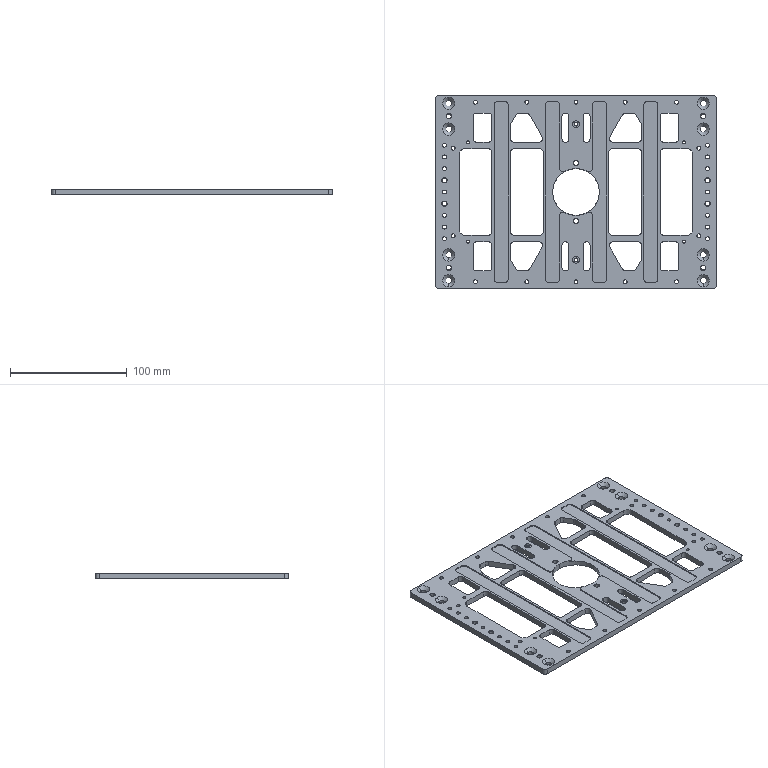NC program | NX | posted with a generic post | part box 240 x 165 x 5 mm
Lines 11987 to 12487 of 12487:
(刀补14 , TOOL : D10JING)
N23870 T14 M6
N23872 G54
N23874 G17 G0 G90 X-64.983 Y7.189 S9500 M3
N23876 G43 Z30. H14
N23878 Z1.
N23880 G94 G1 Y0.098 Z-0.9 F1500.
N23882 G41 X-65. Y0. D14
N23884 Y-72.5
N23886 X-63.
N23888 Y72.5
N23890 X-65.
N23892 Y0.
N23894 G3 X-64.5 Y-0.866 R1.
N23896 G40
N23898 G1 X-64.406 Y-0.9
N23900 Z0.1
N23902 G0 Z30.
N23904 X-18.906 Y1.766
N23906 Z0.1
N23908 G1 Z-0.9
N23910 G41 X-19. Y1.732
N23912 X-20.5 Y0.866
N23914 G3 X-21. Y0. R1.
N23916 G1 Y-72.5
N23918 X-19.
N23920 Y-20.199
N23922 G2 X-7.174 Y-13.173 R8.
N23924 G3 X7.174 Y-13.173 R15.
N23926 G2 X19. Y-20.199 R8.
N23928 G1 Y-72.5
N23930 X21.
N23932 Y72.5
N23934 X19.
N23936 Y20.199
N23938 G2 X7.174 Y13.173 R8.
N23940 G3 X-7.174 Y13.173 R15.
N23942 G2 X-19. Y20.199 R8.
N23944 G1 Y72.5
N23946 X-21.
N23948 Y0.
N23950 G3 X-20.5 Y-0.866 R1.
N23952 G1 X-19. Y-1.732
N23954 G40
N23956 X-18.906 Y-1.766
N23958 Z0.1
N23960 G0 Z30.
N23962 X64.983 Y-7.189
N23964 Z1.
N23966 G1 Y-0.098 Z-0.9
N23968 G41 X65. Y0.
N23970 Y72.5
N23972 X63.
N23974 Y-72.5
N23976 X65.
N23978 Y0.
N23980 G3 X64.5 Y0.866 R1.
N23982 G40
N23984 G1 X64.406 Y0.9
N23986 Z0.1
N23988 G0 Z30.
N23990 M5
(刀补 , TOOL : D3)
N23992 T17 M6
N23994 G54
N23996 G17 G0 G90 X-108.75 Y-64.75 S9500 M3
N23998 G43 Z30. H17
N24000 Z0.5
N24002 G41 G94 G1 X-108.723 Y-64.846 F1250. D17
N24004 G3 X-108.3 Y-64.75 R0.222
N24006 X-108.3 Y-64.75 Z-0.5 I-0.45 J0.
N24008 X-108.3 Y-64.75 Z-1.5 I-0.45 J0.
N24010 X-108.3 Y-64.75 Z-2.5 I-0.45 J0.
N24012 X-108.3 Y-64.75 Z-3.5 I-0.45 J0.
N24014 X-108.3 Y-64.75 Z-4.5 I-0.45 J0.
N24016 X-109.2 Y-64.75 Z-5. I-0.45 J0.
N24018 X-108.75 Y-65.2 R0.45
N24020 X-109.2 Y-64.75 R-0.45
N24022 X-108.777 Y-64.846 R0.222
N24024 G40
N24026 G1 X-108.75 Y-64.75
N24028 G0 Z30.
N24030 X-112.5 Y-10.
N24032 Z0.5
N24034 G41 G1 X-112.473 Y-10.096
N24036 G3 X-112.05 Y-10. R0.222
N24038 X-112.05 Y-10. Z-0.5 I-0.45 J0.
N24040 X-112.05 Y-10. Z-1.5 I-0.45 J0.
N24042 X-112.05 Y-10. Z-2.5 I-0.45 J0.
N24044 X-112.05 Y-10. Z-3.5 I-0.45 J0.
N24046 X-112.05 Y-10. Z-4.5 I-0.45 J0.
N24048 X-112.95 Y-10. Z-5. I-0.45 J0.
N24050 X-112.5 Y-10.45 R0.45
N24052 X-112.95 Y-10. R-0.45
N24054 X-112.527 Y-10.096 R0.222
N24056 G40
N24058 G1 X-112.5 Y-10.
N24060 G0 Z30.
N24062 Y10.
N24064 Z0.5
N24066 G41 G1 X-112.473 Y9.904
N24068 G3 X-112.05 Y10. R0.222
N24070 X-112.05 Y10. Z-0.5 I-0.45 J0.
N24072 X-112.05 Y10. Z-1.5 I-0.45 J0.
N24074 X-112.05 Y10. Z-2.5 I-0.45 J0.
N24076 X-112.05 Y10. Z-3.5 I-0.45 J0.
N24078 X-112.05 Y10. Z-4.5 I-0.45 J0.
N24080 X-112.95 Y10. Z-5. I-0.45 J0.
N24082 X-112.5 Y9.55 R0.45
N24084 X-112.95 Y10. R-0.45
N24086 X-112.527 Y9.904 R0.222
N24088 G40
N24090 G1 X-112.5 Y10.
N24092 G0 Z30.
N24094 X0. Y25.
N24096 Z0.5
N24098 G41 G1 X0.027 Y24.904
N24100 G3 X0.45 Y25. R0.222
N24102 X0.45 Y25. Z-0.5 I-0.45 J0.
N24104 X0.45 Y25. Z-1.5 I-0.45 J0.
N24106 X0.45 Y25. Z-2.5 I-0.45 J0.
N24108 X0.45 Y25. Z-3.5 I-0.45 J0.
N24110 X0.45 Y25. Z-4.5 I-0.45 J0.
N24112 X-0.45 Y25. Z-5. I-0.45 J0.
N24114 X0. Y24.55 R0.45
N24116 X-0.45 Y25. R-0.45
N24118 X-0.027 Y24.904 R0.222
N24120 G40
N24122 G1 X0. Y25.
N24124 G0 Z30.
N24126 Y-25.
N24128 Z0.5
N24130 G41 G1 X0.027 Y-25.096
N24132 G3 X0.45 Y-25. R0.222
N24134 X0.45 Y-25. Z-0.5 I-0.45 J0.
N24136 X0.45 Y-25. Z-1.5 I-0.45 J0.
N24138 X0.45 Y-25. Z-2.5 I-0.45 J0.
N24140 X0.45 Y-25. Z-3.5 I-0.45 J0.
N24142 X0.45 Y-25. Z-4.5 I-0.45 J0.
N24144 X-0.45 Y-25. Z-5. I-0.45 J0.
N24146 X0. Y-25.45 R0.45
N24148 X-0.45 Y-25. R-0.45
N24150 X-0.027 Y-25.096 R0.222
N24152 G40
N24154 G1 X0. Y-25.
N24156 G0 Z30.
N24158 X108.75 Y-64.75
N24160 Z0.5
N24162 G41 G1 X108.777 Y-64.846
N24164 G3 X109.2 Y-64.75 R0.222
N24166 X109.2 Y-64.75 Z-0.5 I-0.45 J0.
N24168 X109.2 Y-64.75 Z-1.5 I-0.45 J0.
N24170 X109.2 Y-64.75 Z-2.5 I-0.45 J0.
N24172 X109.2 Y-64.75 Z-3.5 I-0.45 J0.
N24174 X109.2 Y-64.75 Z-4.5 I-0.45 J0.
N24176 X108.3 Y-64.75 Z-5. I-0.45 J0.
N24178 X108.75 Y-65.2 R0.45
N24180 X108.3 Y-64.75 R-0.45
N24182 X108.723 Y-64.846 R0.222
N24184 G40
N24186 G1 X108.75 Y-64.75
N24188 G0 Z30.
N24190 X112.5 Y-10.
N24192 Z0.5
N24194 G41 G1 X112.527 Y-10.096
N24196 G3 X112.95 Y-10. R0.222
N24198 X112.95 Y-10. Z-0.5 I-0.45 J0.
N24200 X112.95 Y-10. Z-1.5 I-0.45 J0.
N24202 X112.95 Y-10. Z-2.5 I-0.45 J0.
N24204 X112.95 Y-10. Z-3.5 I-0.45 J0.
N24206 X112.95 Y-10. Z-4.5 I-0.45 J0.
N24208 X112.05 Y-10. Z-5. I-0.45 J0.
N24210 X112.5 Y-10.45 R0.45
N24212 X112.05 Y-10. R-0.45
N24214 X112.473 Y-10.096 R0.222
N24216 G40
N24218 G1 X112.5 Y-10.
N24220 G0 Z30.
N24222 Y10.
N24224 Z0.5
N24226 G41 G1 X112.527 Y9.904
N24228 G3 X112.95 Y10. R0.222
N24230 X112.95 Y10. Z-0.5 I-0.45 J0.
N24232 X112.95 Y10. Z-1.5 I-0.45 J0.
N24234 X112.95 Y10. Z-2.5 I-0.45 J0.
N24236 X112.95 Y10. Z-3.5 I-0.45 J0.
N24238 X112.95 Y10. Z-4.5 I-0.45 J0.
N24240 X112.05 Y10. Z-5. I-0.45 J0.
N24242 X112.5 Y9.55 R0.45
N24244 X112.05 Y10. R-0.45
N24246 X112.473 Y9.904 R0.222
N24248 G40
N24250 G1 X112.5 Y10.
N24252 G0 Z30.
N24254 X108.75 Y64.75
N24256 Z0.5
N24258 G41 G1 X108.777 Y64.654
N24260 G3 X109.2 Y64.75 R0.222
N24262 X109.2 Y64.75 Z-0.5 I-0.45 J0.
N24264 X109.2 Y64.75 Z-1.5 I-0.45 J0.
N24266 X109.2 Y64.75 Z-2.5 I-0.45 J0.
N24268 X109.2 Y64.75 Z-3.5 I-0.45 J0.
N24270 X109.2 Y64.75 Z-4.5 I-0.45 J0.
N24272 X108.3 Y64.75 Z-5. I-0.45 J0.
N24274 X108.75 Y64.3 R0.45
N24276 X108.3 Y64.75 R-0.45
N24278 X108.723 Y64.654 R0.222
N24280 G40
N24282 G1 X108.75 Y64.75
N24284 G0 Z30.
N24286 M5
(ZLEVEL_PROFILE_COPY_1 , TOOL : D10JING)
N24288 T14 M6
N24290 G54
N24292 G17 G0 G90 X-31.007 Y87.5 S9500 M3
N24294 G43 Z30. H14
N24296 Z-2.9
N24298 G94 G1 X0. Z-4.525 F1000.
N24300 X117. F1200.
N24302 G2 X125. Y79.5 R8.
N24304 G1 Y-79.5
N24306 G2 X117. Y-87.5 R8.
N24308 G1 X-117.
N24310 G2 X-125. Y-79.5 R8.
N24312 G1 Y79.5
N24314 G2 X-117. Y87.5 R8.
N24316 G1 X0.
N24318 X117. Z-4.542
N24320 X117.628 Y87.475 Z-4.543
N24322 X118.251 Y87.402
N24324 X118.868 Y87.279
N24326 X119.472 Y87.108
N24328 X120.061 Y86.891
N24330 X120.632 Y86.628
N24332 X121.18 Y86.321
N24334 X121.702 Y85.972
N24336 X122.196 Y85.583
N24338 X122.657 Y85.157
N24340 X123.083 Y84.696 Z-4.544
N24342 X123.472 Y84.202
N24344 X123.821 Y83.68
N24346 X124.128 Y83.132
N24348 X124.391 Y82.561
N24350 X124.608 Y81.972
N24352 X124.779 Y81.368
N24354 X124.902 Y80.751
N24356 X124.975 Y80.128
N24358 X125. Y79.5
N24360 Y-79.5 Z-4.568
N24362 X124.975 Y-80.128
N24364 X124.902 Y-80.751
N24366 X124.779 Y-81.368
N24368 X124.608 Y-81.972 Z-4.569
N24370 X124.391 Y-82.561
N24372 X124.128 Y-83.132
N24374 X123.821 Y-83.68
N24376 X123.472 Y-84.202
N24378 X123.083 Y-84.696
N24380 X122.657 Y-85.157
N24382 X122.196 Y-85.583
N24384 X121.702 Y-85.972
N24386 X121.18 Y-86.321
N24388 X120.632 Y-86.628
N24390 X120.061 Y-86.891 Z-4.57
N24392 X119.472 Y-87.108
N24394 X118.868 Y-87.279
N24396 X118.251 Y-87.402
N24398 X117.628 Y-87.475
N24400 X117. Y-87.5
N24402 X-117. Z-4.605
N24404 X-117.628 Y-87.475
N24406 X-118.251 Y-87.402
N24408 X-118.868 Y-87.279
N24410 X-119.472 Y-87.108
N24412 X-120.061 Y-86.891
N24414 X-120.632 Y-86.628 Z-4.606
N24416 X-121.18 Y-86.321
N24418 X-121.702 Y-85.972
N24420 X-122.196 Y-85.583
N24422 X-122.657 Y-85.157
N24424 X-123.083 Y-84.696
N24426 X-123.472 Y-84.202
N24428 X-123.821 Y-83.68
N24430 X-124.128 Y-83.132
N24432 X-124.391 Y-82.561
N24434 X-124.608 Y-81.972
N24436 X-124.779 Y-81.368 Z-4.607
N24438 X-124.902 Y-80.751
N24440 X-124.975 Y-80.128
N24442 X-125. Y-79.5
N24444 Y79.5 Z-4.631
N24446 X-124.975 Y80.128
N24448 X-124.902 Y80.751
N24450 X-124.779 Y81.368
N24452 X-124.608 Y81.972
N24454 X-124.391 Y82.561
N24456 X-124.128 Y83.132
N24458 X-123.821 Y83.68
N24460 X-123.472 Y84.202
N24462 X-123.083 Y84.696
N24464 X-122.657 Y85.157 Z-4.632
N24466 X-122.196 Y85.583
N24468 X-121.702 Y85.972
N24470 X-121.18 Y86.321
N24472 X-120.632 Y86.628
N24474 X-120.061 Y86.891
N24476 X-119.472 Y87.108
N24478 X-118.868 Y87.279
N24480 X-118.251 Y87.402
N24482 X-117.628 Y87.475
N24484 X-117. Y87.5 Z-4.633
N24486 X0. Z-4.65
N24488 X117. Z-4.667
N24490 X117.628 Y87.475 Z-4.668
N24492 X118.251 Y87.402
N24494 X118.868 Y87.279
N24496 X119.472 Y87.108
N24498 X120.061 Y86.891
N24500 X120.632 Y86.628
N24502 X121.18 Y86.321
N24504 X121.702 Y85.972
N24506 X122.196 Y85.583
N24508 X122.657 Y85.157
N24510 X123.083 Y84.696 Z-4.669
N24512 X123.472 Y84.202
N24514 X123.821 Y83.68
N24516 X124.128 Y83.132
N24518 X124.391 Y82.561
N24520 X124.608 Y81.972
N24522 X124.779 Y81.368
N24524 X124.902 Y80.751
N24526 X124.975 Y80.128
N24528 X125. Y79.5
N24530 Y-79.5 Z-4.693
N24532 X124.975 Y-80.128
N24534 X124.902 Y-80.751
N24536 X124.779 Y-81.368
N24538 X124.608 Y-81.972 Z-4.694
N24540 X124.391 Y-82.561
N24542 X124.128 Y-83.132
N24544 X123.821 Y-83.68
N24546 X123.472 Y-84.202
N24548 X123.083 Y-84.696
N24550 X122.657 Y-85.157
N24552 X122.196 Y-85.583
N24554 X121.702 Y-85.972
N24556 X121.18 Y-86.321
N24558 X120.632 Y-86.628
N24560 X120.061 Y-86.891 Z-4.695
N24562 X119.472 Y-87.108
N24564 X118.868 Y-87.279
N24566 X118.251 Y-87.402
N24568 X117.628 Y-87.475
N24570 X117. Y-87.5
N24572 X-117. Z-4.73
N24574 X-117.628 Y-87.475
N24576 X-118.251 Y-87.402
N24578 X-118.868 Y-87.279
N24580 X-119.472 Y-87.108
N24582 X-120.061 Y-86.891
N24584 X-120.632 Y-86.628 Z-4.731
N24586 X-121.18 Y-86.321
N24588 X-121.702 Y-85.972
N24590 X-122.196 Y-85.583
N24592 X-122.657 Y-85.157
N24594 X-123.083 Y-84.696
N24596 X-123.472 Y-84.202
N24598 X-123.821 Y-83.68
N24600 X-124.128 Y-83.132
N24602 X-124.391 Y-82.561
N24604 X-124.608 Y-81.972
N24606 X-124.779 Y-81.368 Z-4.732
N24608 X-124.902 Y-80.751
N24610 X-124.975 Y-80.128
N24612 X-125. Y-79.5
N24614 Y79.5 Z-4.756
N24616 X-124.975 Y80.128
N24618 X-124.902 Y80.751
N24620 X-124.779 Y81.368
N24622 X-124.608 Y81.972
N24624 X-124.391 Y82.561
N24626 X-124.128 Y83.132
N24628 X-123.821 Y83.68
N24630 X-123.472 Y84.202
N24632 X-123.083 Y84.696
N24634 X-122.657 Y85.157 Z-4.757
N24636 X-122.196 Y85.583
N24638 X-121.702 Y85.972
N24640 X-121.18 Y86.321
N24642 X-120.632 Y86.628
N24644 X-120.061 Y86.891
N24646 X-119.472 Y87.108
N24648 X-118.868 Y87.279
N24650 X-118.251 Y87.402
N24652 X-117.628 Y87.475
N24654 X-117. Y87.5 Z-4.758
N24656 X0. Z-4.775
N24658 X117. Z-4.792
N24660 X117.628 Y87.475 Z-4.793
N24662 X118.251 Y87.402
N24664 X118.868 Y87.279
N24666 X119.472 Y87.108
N24668 X120.061 Y86.891
N24670 X120.632 Y86.628
N24672 X121.18 Y86.321
N24674 X121.702 Y85.972
N24676 X122.196 Y85.583
N24678 X122.657 Y85.157
N24680 X123.083 Y84.696 Z-4.794
N24682 X123.472 Y84.202
N24684 X123.821 Y83.68
N24686 X124.128 Y83.132
N24688 X124.391 Y82.561
N24690 X124.608 Y81.972
N24692 X124.779 Y81.368
N24694 X124.902 Y80.751
N24696 X124.975 Y80.128
N24698 X125. Y79.5
N24700 Y-79.5 Z-4.818
N24702 X124.975 Y-80.128
N24704 X124.902 Y-80.751
N24706 X124.779 Y-81.368
N24708 X124.608 Y-81.972 Z-4.819
N24710 X124.391 Y-82.561
N24712 X124.128 Y-83.132
N24714 X123.821 Y-83.68
N24716 X123.472 Y-84.202
N24718 X123.083 Y-84.696
N24720 X122.657 Y-85.157
N24722 X122.196 Y-85.583
N24724 X121.702 Y-85.972
N24726 X121.18 Y-86.321
N24728 X120.632 Y-86.628
N24730 X120.061 Y-86.891 Z-4.82
N24732 X119.472 Y-87.108
N24734 X118.868 Y-87.279
N24736 X118.251 Y-87.402
N24738 X117.628 Y-87.475
N24740 X117. Y-87.5
N24742 X-117. Z-4.855
N24744 X-117.628 Y-87.475
N24746 X-118.251 Y-87.402
N24748 X-118.868 Y-87.279
N24750 X-119.472 Y-87.108
N24752 X-120.061 Y-86.891
N24754 X-120.632 Y-86.628 Z-4.856
N24756 X-121.18 Y-86.321
N24758 X-121.702 Y-85.972
N24760 X-122.196 Y-85.583
N24762 X-122.657 Y-85.157
N24764 X-123.083 Y-84.696
N24766 X-123.472 Y-84.202
N24768 X-123.821 Y-83.68
N24770 X-124.128 Y-83.132
N24772 X-124.391 Y-82.561
N24774 X-124.608 Y-81.972
N24776 X-124.779 Y-81.368 Z-4.857
N24778 X-124.902 Y-80.751
N24780 X-124.975 Y-80.128
N24782 X-125. Y-79.5
N24784 Y79.5 Z-4.881
N24786 X-124.975 Y80.128
N24788 X-124.902 Y80.751
N24790 X-124.779 Y81.368
N24792 X-124.608 Y81.972
N24794 X-124.391 Y82.561
N24796 X-124.128 Y83.132
N24798 X-123.821 Y83.68
N24800 X-123.472 Y84.202
N24802 X-123.083 Y84.696
N24804 X-122.657 Y85.157 Z-4.882
N24806 X-122.196 Y85.583
N24808 X-121.702 Y85.972
N24810 X-121.18 Y86.321
N24812 X-120.632 Y86.628
N24814 X-120.061 Y86.891
N24816 X-119.472 Y87.108
N24818 X-118.868 Y87.279
N24820 X-118.251 Y87.402
N24822 X-117.628 Y87.475
N24824 X-117. Y87.5 Z-4.883
N24826 X0. Z-4.9
N24828 X117.
N24830 G2 X125. Y79.5 R8.
N24832 G1 Y-79.5
N24834 G2 X117. Y-87.5 R8.
N24836 G1 X-117.
N24838 G2 X-125. Y-79.5 R8.
N24840 G1 Y79.5
N24842 G2 X-117. Y87.5 R8.
N24844 G1 X0.
N24846 Z-3.4
N24848 G0 Z30.
N24850 M5
N24852 M2